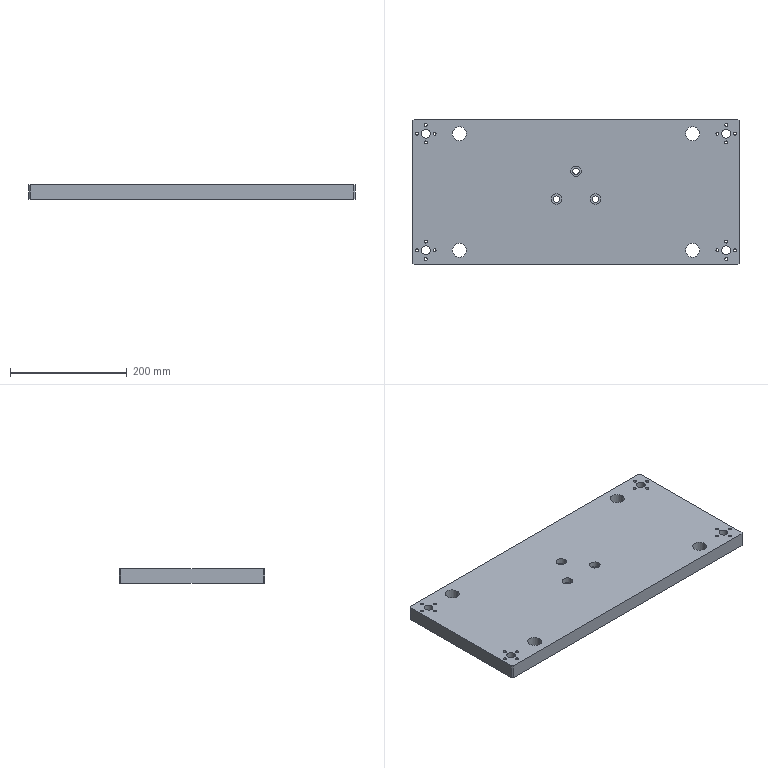Part | STEP file | Lifting Top Plate | 1 solid | 73 faces | box 560 x 250 x 25 mm | volume 3417013 mm3 | cylinder 60 | plane 13 | commonest cylinder face diameters 5 x32 15 x8 24 x8 11 x6 18 x6